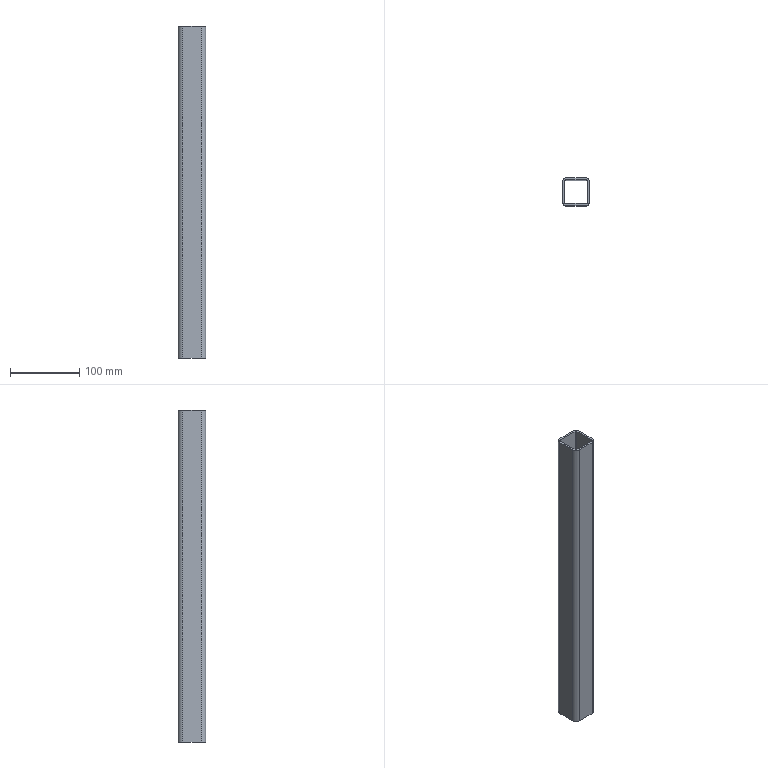Part | SolidWorks | features Fillet 2, Extrusion 1 | 1 solid | 18 faces | box 40 x 40 x 479.48 mm | volume 194368 mm3 | plane 10 | cylinder 8 | commonest cylinder face diameters 4 x4 14 x4
STEP:
#1=CARTESIAN_POINT('',(20.,-13.,479.48));
#2=VERTEX_POINT('',#1);
#3=CARTESIAN_POINT('',(20.,13.,479.48));
#4=VERTEX_POINT('',#3);
#5=CARTESIAN_POINT('',(20.,20.,479.48));
#6=DIRECTION('',(0.,1.,0.));
#7=VECTOR('',#6,1000.);
#8=LINE('',#5,#7);
#9=EDGE_CURVE('',#2,#4,#8,.T.);
#10=ORIENTED_EDGE('',*,*,#9,.T.);
#11=CARTESIAN_POINT('',(13.,20.,479.48));
#12=VERTEX_POINT('',#11);
#13=CARTESIAN_POINT('',(13.,13.,479.48));
#14=DIRECTION('',(0.,0.,1.));
#15=DIRECTION('',(1.,0.,0.));
#16=AXIS2_PLACEMENT_3D('',#13,#14,#15);
#17=CIRCLE('',#16,7.);
#18=EDGE_CURVE('',#4,#12,#17,.T.);
#19=ORIENTED_EDGE('',*,*,#18,.T.);
#20=CARTESIAN_POINT('',(-13.,20.,479.48));
#21=VERTEX_POINT('',#20);
#22=CARTESIAN_POINT('',(-20.,20.,479.48));
#23=DIRECTION('',(-1.,0.,0.));
#24=VECTOR('',#23,1000.);
#25=LINE('',#22,#24);
#26=EDGE_CURVE('',#12,#21,#25,.T.);
#27=ORIENTED_EDGE('',*,*,#26,.T.);
#28=CARTESIAN_POINT('',(-20.,13.,479.48));
#29=VERTEX_POINT('',#28);
#30=CARTESIAN_POINT('',(-13.,13.,479.48));
#31=DIRECTION('',(0.,0.,1.));
#32=DIRECTION('',(1.,0.,0.));
#33=AXIS2_PLACEMENT_3D('',#30,#31,#32);
#34=CIRCLE('',#33,7.);
#35=EDGE_CURVE('',#21,#29,#34,.T.);
#36=ORIENTED_EDGE('',*,*,#35,.T.);
#37=CARTESIAN_POINT('',(-20.,-13.,479.48));
#38=VERTEX_POINT('',#37);
#39=CARTESIAN_POINT('',(-20.,20.,479.48));
#40=DIRECTION('',(0.,-1.,0.));
#41=VECTOR('',#40,1000.);
#42=LINE('',#39,#41);
#43=EDGE_CURVE('',#29,#38,#42,.T.);
#44=ORIENTED_EDGE('',*,*,#43,.T.);
#45=CARTESIAN_POINT('',(-13.,-20.,479.48));
#46=VERTEX_POINT('',#45);
#47=CARTESIAN_POINT('',(-13.,-13.,479.48));
#48=DIRECTION('',(0.,0.,1.));
#49=DIRECTION('',(1.,0.,0.));
#50=AXIS2_PLACEMENT_3D('',#47,#48,#49);
#51=CIRCLE('',#50,7.);
#52=EDGE_CURVE('',#38,#46,#51,.T.);
#53=ORIENTED_EDGE('',*,*,#52,.T.);
#54=CARTESIAN_POINT('',(13.,-20.,479.48));
#55=VERTEX_POINT('',#54);
#56=CARTESIAN_POINT('',(-20.,-20.,479.48));
#57=DIRECTION('',(1.,0.,0.));
#58=VECTOR('',#57,1000.);
#59=LINE('',#56,#58);
#60=EDGE_CURVE('',#46,#55,#59,.T.);
#61=ORIENTED_EDGE('',*,*,#60,.T.);
#62=CARTESIAN_POINT('',(13.,-13.,479.48));
#63=DIRECTION('',(0.,0.,1.));
#64=DIRECTION('',(1.,0.,0.));
#65=AXIS2_PLACEMENT_3D('',#62,#63,#64);
#66=CIRCLE('',#65,7.);
#67=EDGE_CURVE('',#55,#2,#66,.T.);
#68=ORIENTED_EDGE('',*,*,#67,.T.);
#69=EDGE_LOOP('',(#10,#19,#27,#36,#44,#53,#61,#68));
#70=FACE_OUTER_BOUND('',#69,.T.);
#71=CARTESIAN_POINT('',(15.,17.,479.48));
#72=VERTEX_POINT('',#71);
#73=CARTESIAN_POINT('',(-15.,17.,479.48));
#74=VERTEX_POINT('',#73);
#75=CARTESIAN_POINT('',(-17.,17.,479.48));
#76=DIRECTION('',(-1.,0.,0.));
#77=VECTOR('',#76,1000.);
#78=LINE('',#75,#77);
#79=EDGE_CURVE('',#72,#74,#78,.T.);
#80=ORIENTED_EDGE('',*,*,#79,.F.);
#81=CARTESIAN_POINT('',(17.,15.,479.48));
#82=VERTEX_POINT('',#81);
#83=CARTESIAN_POINT('',(15.,15.,479.48));
#84=DIRECTION('',(0.,0.,-1.));
#85=DIRECTION('',(1.,0.,0.));
#86=AXIS2_PLACEMENT_3D('',#83,#84,#85);
#87=CIRCLE('',#86,2.);
#88=EDGE_CURVE('',#72,#82,#87,.T.);
#89=ORIENTED_EDGE('',*,*,#88,.T.);
#90=CARTESIAN_POINT('',(17.,-15.,479.48));
#91=VERTEX_POINT('',#90);
#92=CARTESIAN_POINT('',(17.,17.,479.48));
#93=DIRECTION('',(0.,1.,0.));
#94=VECTOR('',#93,1000.);
#95=LINE('',#92,#94);
#96=EDGE_CURVE('',#91,#82,#95,.T.);
#97=ORIENTED_EDGE('',*,*,#96,.F.);
#98=CARTESIAN_POINT('',(15.,-17.,479.48));
#99=VERTEX_POINT('',#98);
#100=CARTESIAN_POINT('',(15.,-15.,479.48));
#101=DIRECTION('',(0.,0.,-1.));
#102=DIRECTION('',(1.,0.,0.));
#103=AXIS2_PLACEMENT_3D('',#100,#101,#102);
#104=CIRCLE('',#103,2.);
#105=EDGE_CURVE('',#91,#99,#104,.T.);
#106=ORIENTED_EDGE('',*,*,#105,.T.);
#107=CARTESIAN_POINT('',(-15.,-17.,479.48));
#108=VERTEX_POINT('',#107);
#109=CARTESIAN_POINT('',(-17.,-17.,479.48));
#110=DIRECTION('',(1.,0.,0.));
#111=VECTOR('',#110,1000.);
#112=LINE('',#109,#111);
#113=EDGE_CURVE('',#108,#99,#112,.T.);
#114=ORIENTED_EDGE('',*,*,#113,.F.);
#115=CARTESIAN_POINT('',(-17.,-15.,479.48));
#116=VERTEX_POINT('',#115);
#117=CARTESIAN_POINT('',(-15.,-15.,479.48));
#118=DIRECTION('',(0.,0.,-1.));
#119=DIRECTION('',(1.,0.,0.));
#120=AXIS2_PLACEMENT_3D('',#117,#118,#119);
#121=CIRCLE('',#120,2.);
#122=EDGE_CURVE('',#108,#116,#121,.T.);
#123=ORIENTED_EDGE('',*,*,#122,.T.);
#124=CARTESIAN_POINT('',(-17.,15.,479.48));
#125=VERTEX_POINT('',#124);
#126=CARTESIAN_POINT('',(-17.,17.,479.48));
#127=DIRECTION('',(0.,-1.,0.));
#128=VECTOR('',#127,1000.);
#129=LINE('',#126,#128);
#130=EDGE_CURVE('',#125,#116,#129,.T.);
#131=ORIENTED_EDGE('',*,*,#130,.F.);
#132=CARTESIAN_POINT('',(-15.,15.,479.48));
#133=DIRECTION('',(0.,0.,-1.));
#134=DIRECTION('',(1.,0.,0.));
#135=AXIS2_PLACEMENT_3D('',#132,#133,#134);
#136=CIRCLE('',#135,2.);
#137=EDGE_CURVE('',#125,#74,#136,.T.);
#138=ORIENTED_EDGE('',*,*,#137,.T.);
#139=EDGE_LOOP('',(#80,#89,#97,#106,#114,#123,#131,#138));
#140=FACE_BOUND('',#139,.T.);
#141=CARTESIAN_POINT('',(0.,0.,479.48));
#142=DIRECTION('',(0.,0.,1.));
#143=DIRECTION('',(1.,0.,0.));
#144=AXIS2_PLACEMENT_3D('',#141,#142,#143);
#145=PLANE('',#144);
#146=ADVANCED_FACE('',(#70,#140),#145,.T.);
#147=CARTESIAN_POINT('',(13.,20.,0.));
#148=VERTEX_POINT('',#147);
#149=CARTESIAN_POINT('',(-13.,20.,0.));
#150=VERTEX_POINT('',#149);
#151=CARTESIAN_POINT('',(-20.,20.,0.));
#152=DIRECTION('',(-1.,0.,0.));
#153=VECTOR('',#152,1000.);
#154=LINE('',#151,#153);
#155=EDGE_CURVE('',#148,#150,#154,.T.);
#156=ORIENTED_EDGE('',*,*,#155,.F.);
#157=CARTESIAN_POINT('',(20.,13.,0.));
#158=VERTEX_POINT('',#157);
#159=CARTESIAN_POINT('',(13.,13.,0.));
#160=DIRECTION('',(0.,0.,-1.));
#161=DIRECTION('',(1.,0.,0.));
#162=AXIS2_PLACEMENT_3D('',#159,#160,#161);
#163=CIRCLE('',#162,7.);
#164=EDGE_CURVE('',#148,#158,#163,.T.);
#165=ORIENTED_EDGE('',*,*,#164,.T.);
#166=CARTESIAN_POINT('',(20.,-13.,0.));
#167=VERTEX_POINT('',#166);
#168=CARTESIAN_POINT('',(20.,20.,0.));
#169=DIRECTION('',(0.,1.,0.));
#170=VECTOR('',#169,1000.);
#171=LINE('',#168,#170);
#172=EDGE_CURVE('',#167,#158,#171,.T.);
#173=ORIENTED_EDGE('',*,*,#172,.F.);
#174=CARTESIAN_POINT('',(13.,-20.,0.));
#175=VERTEX_POINT('',#174);
#176=CARTESIAN_POINT('',(13.,-13.,0.));
#177=DIRECTION('',(0.,0.,-1.));
#178=DIRECTION('',(1.,0.,0.));
#179=AXIS2_PLACEMENT_3D('',#176,#177,#178);
#180=CIRCLE('',#179,7.);
#181=EDGE_CURVE('',#167,#175,#180,.T.);
#182=ORIENTED_EDGE('',*,*,#181,.T.);
#183=CARTESIAN_POINT('',(-13.,-20.,0.));
#184=VERTEX_POINT('',#183);
#185=CARTESIAN_POINT('',(-20.,-20.,0.));
#186=DIRECTION('',(1.,0.,0.));
#187=VECTOR('',#186,1000.);
#188=LINE('',#185,#187);
#189=EDGE_CURVE('',#184,#175,#188,.T.);
#190=ORIENTED_EDGE('',*,*,#189,.F.);
#191=CARTESIAN_POINT('',(-20.,-13.,0.));
#192=VERTEX_POINT('',#191);
#193=CARTESIAN_POINT('',(-13.,-13.,0.));
#194=DIRECTION('',(0.,0.,-1.));
#195=DIRECTION('',(1.,0.,0.));
#196=AXIS2_PLACEMENT_3D('',#193,#194,#195);
#197=CIRCLE('',#196,7.);
#198=EDGE_CURVE('',#184,#192,#197,.T.);
#199=ORIENTED_EDGE('',*,*,#198,.T.);
#200=CARTESIAN_POINT('',(-20.,13.,0.));
#201=VERTEX_POINT('',#200);
#202=CARTESIAN_POINT('',(-20.,20.,0.));
#203=DIRECTION('',(0.,-1.,0.));
#204=VECTOR('',#203,1000.);
#205=LINE('',#202,#204);
#206=EDGE_CURVE('',#201,#192,#205,.T.);
#207=ORIENTED_EDGE('',*,*,#206,.F.);
#208=CARTESIAN_POINT('',(-13.,13.,0.));
#209=DIRECTION('',(0.,0.,-1.));
#210=DIRECTION('',(1.,0.,0.));
#211=AXIS2_PLACEMENT_3D('',#208,#209,#210);
#212=CIRCLE('',#211,7.);
#213=EDGE_CURVE('',#201,#150,#212,.T.);
#214=ORIENTED_EDGE('',*,*,#213,.T.);
#215=EDGE_LOOP('',(#156,#165,#173,#182,#190,#199,#207,#214));
#216=FACE_OUTER_BOUND('',#215,.T.);
#217=CARTESIAN_POINT('',(-15.,-17.,0.));
#218=VERTEX_POINT('',#217);
#219=CARTESIAN_POINT('',(15.,-17.,0.));
#220=VERTEX_POINT('',#219);
#221=CARTESIAN_POINT('',(-17.,-17.,0.));
#222=DIRECTION('',(1.,0.,0.));
#223=VECTOR('',#222,1000.);
#224=LINE('',#221,#223);
#225=EDGE_CURVE('',#218,#220,#224,.T.);
#226=ORIENTED_EDGE('',*,*,#225,.T.);
#227=CARTESIAN_POINT('',(17.,-15.,0.));
#228=VERTEX_POINT('',#227);
#229=CARTESIAN_POINT('',(15.,-15.,0.));
#230=DIRECTION('',(0.,0.,1.));
#231=DIRECTION('',(1.,0.,0.));
#232=AXIS2_PLACEMENT_3D('',#229,#230,#231);
#233=CIRCLE('',#232,2.);
#234=EDGE_CURVE('',#220,#228,#233,.T.);
#235=ORIENTED_EDGE('',*,*,#234,.T.);
#236=CARTESIAN_POINT('',(17.,15.,0.));
#237=VERTEX_POINT('',#236);
#238=CARTESIAN_POINT('',(17.,17.,0.));
#239=DIRECTION('',(0.,1.,0.));
#240=VECTOR('',#239,1000.);
#241=LINE('',#238,#240);
#242=EDGE_CURVE('',#228,#237,#241,.T.);
#243=ORIENTED_EDGE('',*,*,#242,.T.);
#244=CARTESIAN_POINT('',(15.,17.,0.));
#245=VERTEX_POINT('',#244);
#246=CARTESIAN_POINT('',(15.,15.,0.));
#247=DIRECTION('',(0.,0.,1.));
#248=DIRECTION('',(1.,0.,0.));
#249=AXIS2_PLACEMENT_3D('',#246,#247,#248);
#250=CIRCLE('',#249,2.);
#251=EDGE_CURVE('',#237,#245,#250,.T.);
#252=ORIENTED_EDGE('',*,*,#251,.T.);
#253=CARTESIAN_POINT('',(-15.,17.,0.));
#254=VERTEX_POINT('',#253);
#255=CARTESIAN_POINT('',(-17.,17.,0.));
#256=DIRECTION('',(-1.,0.,0.));
#257=VECTOR('',#256,1000.);
#258=LINE('',#255,#257);
#259=EDGE_CURVE('',#245,#254,#258,.T.);
#260=ORIENTED_EDGE('',*,*,#259,.T.);
#261=CARTESIAN_POINT('',(-17.,15.,0.));
#262=VERTEX_POINT('',#261);
#263=CARTESIAN_POINT('',(-15.,15.,0.));
#264=DIRECTION('',(0.,0.,1.));
#265=DIRECTION('',(1.,0.,0.));
#266=AXIS2_PLACEMENT_3D('',#263,#264,#265);
#267=CIRCLE('',#266,2.);
#268=EDGE_CURVE('',#254,#262,#267,.T.);
#269=ORIENTED_EDGE('',*,*,#268,.T.);
#270=CARTESIAN_POINT('',(-17.,-15.,0.));
#271=VERTEX_POINT('',#270);
#272=CARTESIAN_POINT('',(-17.,17.,0.));
#273=DIRECTION('',(0.,-1.,0.));
#274=VECTOR('',#273,1000.);
#275=LINE('',#272,#274);
#276=EDGE_CURVE('',#262,#271,#275,.T.);
#277=ORIENTED_EDGE('',*,*,#276,.T.);
#278=CARTESIAN_POINT('',(-15.,-15.,0.));
#279=DIRECTION('',(0.,0.,1.));
#280=DIRECTION('',(1.,0.,0.));
#281=AXIS2_PLACEMENT_3D('',#278,#279,#280);
#282=CIRCLE('',#281,2.);
#283=EDGE_CURVE('',#271,#218,#282,.T.);
#284=ORIENTED_EDGE('',*,*,#283,.T.);
#285=EDGE_LOOP('',(#226,#235,#243,#252,#260,#269,#277,#284));
#286=FACE_BOUND('',#285,.T.);
#287=CARTESIAN_POINT('',(0.,0.,0.));
#288=DIRECTION('',(0.,0.,1.));
#289=DIRECTION('',(1.,0.,0.));
#290=AXIS2_PLACEMENT_3D('',#287,#288,#289);
#291=PLANE('',#290);
#292=ADVANCED_FACE('',(#216,#286),#291,.F.);
#293=ORIENTED_EDGE('',*,*,#172,.T.);
#294=CARTESIAN_POINT('',(20.,13.,479.48));
#295=DIRECTION('',(0.,0.,1.));
#296=VECTOR('',#295,1000.);
#297=LINE('',#294,#296);
#298=EDGE_CURVE('',#158,#4,#297,.T.);
#299=ORIENTED_EDGE('',*,*,#298,.T.);
#300=ORIENTED_EDGE('',*,*,#9,.F.);
#301=CARTESIAN_POINT('',(20.,-13.,479.48));
#302=DIRECTION('',(0.,0.,-1.));
#303=VECTOR('',#302,1000.);
#304=LINE('',#301,#303);
#305=EDGE_CURVE('',#2,#167,#304,.T.);
#306=ORIENTED_EDGE('',*,*,#305,.T.);
#307=EDGE_LOOP('',(#293,#299,#300,#306));
#308=FACE_OUTER_BOUND('',#307,.T.);
#309=CARTESIAN_POINT('',(20.,20.,479.48));
#310=DIRECTION('',(-1.,0.,0.));
#311=DIRECTION('',(0.,0.,1.));
#312=AXIS2_PLACEMENT_3D('',#309,#310,#311);
#313=PLANE('',#312);
#314=ADVANCED_FACE('',(#308),#313,.F.);
#315=ORIENTED_EDGE('',*,*,#26,.F.);
#316=CARTESIAN_POINT('',(13.,20.,479.48));
#317=DIRECTION('',(0.,0.,-1.));
#318=VECTOR('',#317,1000.);
#319=LINE('',#316,#318);
#320=EDGE_CURVE('',#12,#148,#319,.T.);
#321=ORIENTED_EDGE('',*,*,#320,.T.);
#322=ORIENTED_EDGE('',*,*,#155,.T.);
#323=CARTESIAN_POINT('',(-13.,20.,479.48));
#324=DIRECTION('',(0.,0.,1.));
#325=VECTOR('',#324,1000.);
#326=LINE('',#323,#325);
#327=EDGE_CURVE('',#150,#21,#326,.T.);
#328=ORIENTED_EDGE('',*,*,#327,.T.);
#329=EDGE_LOOP('',(#315,#321,#322,#328));
#330=FACE_OUTER_BOUND('',#329,.T.);
#331=CARTESIAN_POINT('',(-20.,20.,479.48));
#332=DIRECTION('',(0.,-1.,0.));
#333=DIRECTION('',(0.,0.,-1.));
#334=AXIS2_PLACEMENT_3D('',#331,#332,#333);
#335=PLANE('',#334);
#336=ADVANCED_FACE('',(#330),#335,.F.);
#337=ORIENTED_EDGE('',*,*,#43,.F.);
#338=CARTESIAN_POINT('',(-20.,13.,479.48));
#339=DIRECTION('',(0.,0.,-1.));
#340=VECTOR('',#339,1000.);
#341=LINE('',#338,#340);
#342=EDGE_CURVE('',#29,#201,#341,.T.);
#343=ORIENTED_EDGE('',*,*,#342,.T.);
#344=ORIENTED_EDGE('',*,*,#206,.T.);
#345=CARTESIAN_POINT('',(-20.,-13.,479.48));
#346=DIRECTION('',(0.,0.,1.));
#347=VECTOR('',#346,1000.);
#348=LINE('',#345,#347);
#349=EDGE_CURVE('',#192,#38,#348,.T.);
#350=ORIENTED_EDGE('',*,*,#349,.T.);
#351=EDGE_LOOP('',(#337,#343,#344,#350));
#352=FACE_OUTER_BOUND('',#351,.T.);
#353=CARTESIAN_POINT('',(-20.,20.,479.48));
#354=DIRECTION('',(1.,0.,0.));
#355=DIRECTION('',(0.,0.,-1.));
#356=AXIS2_PLACEMENT_3D('',#353,#354,#355);
#357=PLANE('',#356);
#358=ADVANCED_FACE('',(#352),#357,.F.);
#359=ORIENTED_EDGE('',*,*,#189,.T.);
#360=CARTESIAN_POINT('',(13.,-20.,479.48));
#361=DIRECTION('',(0.,0.,1.));
#362=VECTOR('',#361,1000.);
#363=LINE('',#360,#362);
#364=EDGE_CURVE('',#175,#55,#363,.T.);
#365=ORIENTED_EDGE('',*,*,#364,.T.);
#366=ORIENTED_EDGE('',*,*,#60,.F.);
#367=CARTESIAN_POINT('',(-13.,-20.,479.48));
#368=DIRECTION('',(0.,0.,-1.));
#369=VECTOR('',#368,1000.);
#370=LINE('',#367,#369);
#371=EDGE_CURVE('',#46,#184,#370,.T.);
#372=ORIENTED_EDGE('',*,*,#371,.T.);
#373=EDGE_LOOP('',(#359,#365,#366,#372));
#374=FACE_OUTER_BOUND('',#373,.T.);
#375=CARTESIAN_POINT('',(-20.,-20.,479.48));
#376=DIRECTION('',(0.,1.,0.));
#377=DIRECTION('',(0.,0.,1.));
#378=AXIS2_PLACEMENT_3D('',#375,#376,#377);
#379=PLANE('',#378);
#380=ADVANCED_FACE('',(#374),#379,.F.);
#381=ORIENTED_EDGE('',*,*,#96,.T.);
#382=CARTESIAN_POINT('',(17.,15.,0.));
#383=DIRECTION('',(0.,0.,-1.));
#384=VECTOR('',#383,1000.);
#385=LINE('',#382,#384);
#386=EDGE_CURVE('',#82,#237,#385,.T.);
#387=ORIENTED_EDGE('',*,*,#386,.T.);
#388=ORIENTED_EDGE('',*,*,#242,.F.);
#389=CARTESIAN_POINT('',(17.,-15.,479.48));
#390=DIRECTION('',(0.,0.,1.));
#391=VECTOR('',#390,1000.);
#392=LINE('',#389,#391);
#393=EDGE_CURVE('',#228,#91,#392,.T.);
#394=ORIENTED_EDGE('',*,*,#393,.T.);
#395=EDGE_LOOP('',(#381,#387,#388,#394));
#396=FACE_OUTER_BOUND('',#395,.T.);
#397=CARTESIAN_POINT('',(17.,17.,479.48));
#398=DIRECTION('',(-1.,0.,0.));
#399=DIRECTION('',(0.,0.,1.));
#400=AXIS2_PLACEMENT_3D('',#397,#398,#399);
#401=PLANE('',#400);
#402=ADVANCED_FACE('',(#396),#401,.T.);
#403=ORIENTED_EDGE('',*,*,#259,.F.);
#404=CARTESIAN_POINT('',(15.,17.,479.48));
#405=DIRECTION('',(0.,0.,1.));
#406=VECTOR('',#405,1000.);
#407=LINE('',#404,#406);
#408=EDGE_CURVE('',#245,#72,#407,.T.);
#409=ORIENTED_EDGE('',*,*,#408,.T.);
#410=ORIENTED_EDGE('',*,*,#79,.T.);
#411=CARTESIAN_POINT('',(-15.,17.,0.));
#412=DIRECTION('',(0.,0.,-1.));
#413=VECTOR('',#412,1000.);
#414=LINE('',#411,#413);
#415=EDGE_CURVE('',#74,#254,#414,.T.);
#416=ORIENTED_EDGE('',*,*,#415,.T.);
#417=EDGE_LOOP('',(#403,#409,#410,#416));
#418=FACE_OUTER_BOUND('',#417,.T.);
#419=CARTESIAN_POINT('',(-17.,17.,479.48));
#420=DIRECTION('',(0.,-1.,0.));
#421=DIRECTION('',(0.,0.,-1.));
#422=AXIS2_PLACEMENT_3D('',#419,#420,#421);
#423=PLANE('',#422);
#424=ADVANCED_FACE('',(#418),#423,.T.);
#425=ORIENTED_EDGE('',*,*,#276,.F.);
#426=CARTESIAN_POINT('',(-17.,15.,479.48));
#427=DIRECTION('',(0.,0.,1.));
#428=VECTOR('',#427,1000.);
#429=LINE('',#426,#428);
#430=EDGE_CURVE('',#262,#125,#429,.T.);
#431=ORIENTED_EDGE('',*,*,#430,.T.);
#432=ORIENTED_EDGE('',*,*,#130,.T.);
#433=CARTESIAN_POINT('',(-17.,-15.,0.));
#434=DIRECTION('',(0.,0.,-1.));
#435=VECTOR('',#434,1000.);
#436=LINE('',#433,#435);
#437=EDGE_CURVE('',#116,#271,#436,.T.);
#438=ORIENTED_EDGE('',*,*,#437,.T.);
#439=EDGE_LOOP('',(#425,#431,#432,#438));
#440=FACE_OUTER_BOUND('',#439,.T.);
#441=CARTESIAN_POINT('',(-17.,17.,479.48));
#442=DIRECTION('',(1.,0.,0.));
#443=DIRECTION('',(0.,0.,-1.));
#444=AXIS2_PLACEMENT_3D('',#441,#442,#443);
#445=PLANE('',#444);
#446=ADVANCED_FACE('',(#440),#445,.T.);
#447=ORIENTED_EDGE('',*,*,#225,.F.);
#448=CARTESIAN_POINT('',(-15.,-17.,479.48));
#449=DIRECTION('',(0.,0.,1.));
#450=VECTOR('',#449,1000.);
#451=LINE('',#448,#450);
#452=EDGE_CURVE('',#218,#108,#451,.T.);
#453=ORIENTED_EDGE('',*,*,#452,.T.);
#454=ORIENTED_EDGE('',*,*,#113,.T.);
#455=CARTESIAN_POINT('',(15.,-17.,0.));
#456=DIRECTION('',(0.,0.,-1.));
#457=VECTOR('',#456,1000.);
#458=LINE('',#455,#457);
#459=EDGE_CURVE('',#99,#220,#458,.T.);
#460=ORIENTED_EDGE('',*,*,#459,.T.);
#461=EDGE_LOOP('',(#447,#453,#454,#460));
#462=FACE_OUTER_BOUND('',#461,.T.);
#463=CARTESIAN_POINT('',(-17.,-17.,479.48));
#464=DIRECTION('',(0.,1.,0.));
#465=DIRECTION('',(0.,0.,1.));
#466=AXIS2_PLACEMENT_3D('',#463,#464,#465);
#467=PLANE('',#466);
#468=ADVANCED_FACE('',(#462),#467,.T.);
#469=ORIENTED_EDGE('',*,*,#88,.F.);
#470=ORIENTED_EDGE('',*,*,#408,.F.);
#471=ORIENTED_EDGE('',*,*,#251,.F.);
#472=ORIENTED_EDGE('',*,*,#386,.F.);
#473=EDGE_LOOP('',(#469,#470,#471,#472));
#474=FACE_OUTER_BOUND('',#473,.T.);
#475=CARTESIAN_POINT('',(15.,15.,479.48));
#476=DIRECTION('',(0.,0.,1.));
#477=DIRECTION('',(1.,0.,0.));
#478=AXIS2_PLACEMENT_3D('',#475,#476,#477);
#479=CYLINDRICAL_SURFACE('',#478,2.);
#480=ADVANCED_FACE('',(#474),#479,.F.);
#481=ORIENTED_EDGE('',*,*,#137,.F.);
#482=ORIENTED_EDGE('',*,*,#430,.F.);
#483=ORIENTED_EDGE('',*,*,#268,.F.);
#484=ORIENTED_EDGE('',*,*,#415,.F.);
#485=EDGE_LOOP('',(#481,#482,#483,#484));
#486=FACE_OUTER_BOUND('',#485,.T.);
#487=CARTESIAN_POINT('',(-15.,15.,479.48));
#488=DIRECTION('',(0.,0.,1.));
#489=DIRECTION('',(1.,0.,0.));
#490=AXIS2_PLACEMENT_3D('',#487,#488,#489);
#491=CYLINDRICAL_SURFACE('',#490,2.);
#492=ADVANCED_FACE('',(#486),#491,.F.);
#493=ORIENTED_EDGE('',*,*,#122,.F.);
#494=ORIENTED_EDGE('',*,*,#452,.F.);
#495=ORIENTED_EDGE('',*,*,#283,.F.);
#496=ORIENTED_EDGE('',*,*,#437,.F.);
#497=EDGE_LOOP('',(#493,#494,#495,#496));
#498=FACE_OUTER_BOUND('',#497,.T.);
#499=CARTESIAN_POINT('',(-15.,-15.,479.48));
#500=DIRECTION('',(0.,0.,1.));
#501=DIRECTION('',(1.,0.,0.));
#502=AXIS2_PLACEMENT_3D('',#499,#500,#501);
#503=CYLINDRICAL_SURFACE('',#502,2.);
#504=ADVANCED_FACE('',(#498),#503,.F.);
#505=ORIENTED_EDGE('',*,*,#105,.F.);
#506=ORIENTED_EDGE('',*,*,#393,.F.);
#507=ORIENTED_EDGE('',*,*,#234,.F.);
#508=ORIENTED_EDGE('',*,*,#459,.F.);
#509=EDGE_LOOP('',(#505,#506,#507,#508));
#510=FACE_OUTER_BOUND('',#509,.T.);
#511=CARTESIAN_POINT('',(15.,-15.,479.48));
#512=DIRECTION('',(0.,0.,1.));
#513=DIRECTION('',(1.,0.,0.));
#514=AXIS2_PLACEMENT_3D('',#511,#512,#513);
#515=CYLINDRICAL_SURFACE('',#514,2.);
#516=ADVANCED_FACE('',(#510),#515,.F.);
#517=ORIENTED_EDGE('',*,*,#18,.F.);
#518=ORIENTED_EDGE('',*,*,#298,.F.);
#519=ORIENTED_EDGE('',*,*,#164,.F.);
#520=ORIENTED_EDGE('',*,*,#320,.F.);
#521=EDGE_LOOP('',(#517,#518,#519,#520));
#522=FACE_OUTER_BOUND('',#521,.T.);
#523=CARTESIAN_POINT('',(13.,13.,479.48));
#524=DIRECTION('',(0.,0.,-1.));
#525=DIRECTION('',(-1.,0.,0.));
#526=AXIS2_PLACEMENT_3D('',#523,#524,#525);
#527=CYLINDRICAL_SURFACE('',#526,7.);
#528=ADVANCED_FACE('',(#522),#527,.T.);
#529=ORIENTED_EDGE('',*,*,#67,.F.);
#530=ORIENTED_EDGE('',*,*,#364,.F.);
#531=ORIENTED_EDGE('',*,*,#181,.F.);
#532=ORIENTED_EDGE('',*,*,#305,.F.);
#533=EDGE_LOOP('',(#529,#530,#531,#532));
#534=FACE_OUTER_BOUND('',#533,.T.);
#535=CARTESIAN_POINT('',(13.,-13.,479.48));
#536=DIRECTION('',(0.,0.,-1.));
#537=DIRECTION('',(-1.,0.,0.));
#538=AXIS2_PLACEMENT_3D('',#535,#536,#537);
#539=CYLINDRICAL_SURFACE('',#538,7.);
#540=ADVANCED_FACE('',(#534),#539,.T.);
#541=ORIENTED_EDGE('',*,*,#35,.F.);
#542=ORIENTED_EDGE('',*,*,#327,.F.);
#543=ORIENTED_EDGE('',*,*,#213,.F.);
#544=ORIENTED_EDGE('',*,*,#342,.F.);
#545=EDGE_LOOP('',(#541,#542,#543,#544));
#546=FACE_OUTER_BOUND('',#545,.T.);
#547=CARTESIAN_POINT('',(-13.,13.,479.48));
#548=DIRECTION('',(0.,0.,-1.));
#549=DIRECTION('',(-1.,0.,0.));
#550=AXIS2_PLACEMENT_3D('',#547,#548,#549);
#551=CYLINDRICAL_SURFACE('',#550,7.);
#552=ADVANCED_FACE('',(#546),#551,.T.);
#553=ORIENTED_EDGE('',*,*,#52,.F.);
#554=ORIENTED_EDGE('',*,*,#349,.F.);
#555=ORIENTED_EDGE('',*,*,#198,.F.);
#556=ORIENTED_EDGE('',*,*,#371,.F.);
#557=EDGE_LOOP('',(#553,#554,#555,#556));
#558=FACE_OUTER_BOUND('',#557,.T.);
#559=CARTESIAN_POINT('',(-13.,-13.,479.48));
#560=DIRECTION('',(0.,0.,-1.));
#561=DIRECTION('',(-1.,0.,0.));
#562=AXIS2_PLACEMENT_3D('',#559,#560,#561);
#563=CYLINDRICAL_SURFACE('',#562,7.);
#564=ADVANCED_FACE('',(#558),#563,.T.);
#565=CLOSED_SHELL('',(#146,#292,#314,#336,#358,#380,#402,#424,#446,#468,#480,#492,#504,#516,#528,#540,#552,#564));
#566=MANIFOLD_SOLID_BREP('',#565);
#567=CARTESIAN_POINT('',(0.,0.,0.));
#568=DIRECTION('',(0.,0.,1.));
#569=DIRECTION('',(1.,0.,0.));
#570=AXIS2_PLACEMENT_3D('',#567,#568,#569);
#571=(LENGTH_UNIT()NAMED_UNIT(*)SI_UNIT(.MILLI.,.METRE.));
#572=UNCERTAINTY_MEASURE_WITH_UNIT(LENGTH_MEASURE(0.00001),#571,'','');
#573=(NAMED_UNIT(*)PLANE_ANGLE_UNIT()SI_UNIT($,.RADIAN.));
#574=(NAMED_UNIT(*)SI_UNIT($,.STERADIAN.)SOLID_ANGLE_UNIT());
#575=(GEOMETRIC_REPRESENTATION_CONTEXT(3)GLOBAL_UNCERTAINTY_ASSIGNED_CONTEXT((#572))GLOBAL_UNIT_ASSIGNED_CONTEXT((#571,#573,#574))REPRESENTATION_CONTEXT('',''));
#576=ADVANCED_BREP_SHAPE_REPRESENTATION('',(#566,#570),#575);